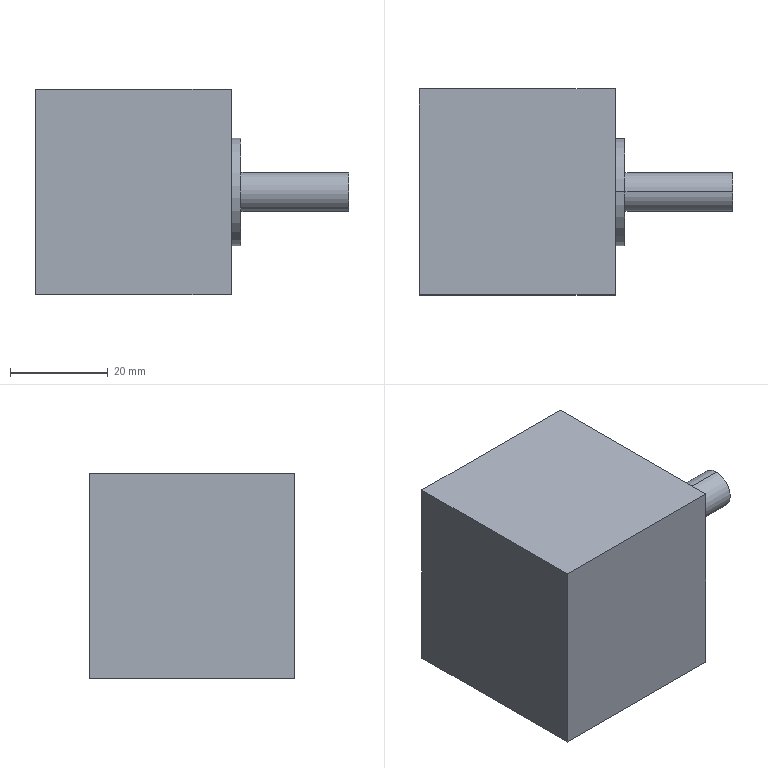Part | SolidWorks | features BaseBody 1 | 1 solid | 36 faces | box 64 x 42 x 42 mm | volume 72019 mm3 | cylinder 20 | plane 16 | commonest cylinder face diameters 3.4 x8 4.3 x8 8 x2 22 x2
STEP:
#1=CARTESIAN_POINT('',(-6.2,-15.5,17.65));
#2=VERTEX_POINT('',#1);
#3=CARTESIAN_POINT('',(-6.2,-15.5,13.35));
#4=VERTEX_POINT('',#3);
#5=CARTESIAN_POINT('',(-6.2,-15.5,15.5));
#6=DIRECTION('',(1.,0.,0.));
#7=DIRECTION('',(0.,0.,-1.));
#8=AXIS2_PLACEMENT_3D('',#5,#6,#7);
#9=CIRCLE('',#8,2.15);
#10=EDGE_CURVE('',#2,#4,#9,.T.);
#11=ORIENTED_EDGE('',*,*,#10,.F.);
#12=CARTESIAN_POINT('',(0.,-15.5,17.65));
#13=VERTEX_POINT('',#12);
#14=CARTESIAN_POINT('',(-6.2,-15.5,17.65));
#15=DIRECTION('',(1.,0.,0.));
#16=VECTOR('',#15,1000.);
#17=LINE('',#14,#16);
#18=EDGE_CURVE('',#2,#13,#17,.T.);
#19=ORIENTED_EDGE('',*,*,#18,.T.);
#20=CARTESIAN_POINT('',(0.,-15.5,13.35));
#21=VERTEX_POINT('',#20);
#22=CARTESIAN_POINT('',(0.,-15.5,15.5));
#23=DIRECTION('',(-1.,0.,0.));
#24=DIRECTION('',(0.,0.,-1.));
#25=AXIS2_PLACEMENT_3D('',#22,#23,#24);
#26=CIRCLE('',#25,2.15);
#27=EDGE_CURVE('',#21,#13,#26,.T.);
#28=ORIENTED_EDGE('',*,*,#27,.F.);
#29=CARTESIAN_POINT('',(-6.2,-15.5,13.35));
#30=DIRECTION('',(1.,0.,0.));
#31=VECTOR('',#30,1000.);
#32=LINE('',#29,#31);
#33=EDGE_CURVE('',#4,#21,#32,.T.);
#34=ORIENTED_EDGE('',*,*,#33,.F.);
#35=EDGE_LOOP('',(#11,#19,#28,#34));
#36=FACE_OUTER_BOUND('',#35,.T.);
#37=CARTESIAN_POINT('',(-6.2,-15.5,15.5));
#38=DIRECTION('',(1.,0.,0.));
#39=DIRECTION('',(0.,0.,-1.));
#40=AXIS2_PLACEMENT_3D('',#37,#38,#39);
#41=CYLINDRICAL_SURFACE('',#40,2.15);
#42=ADVANCED_FACE('',(#36),#41,.F.);
#43=CARTESIAN_POINT('',(0.,0.,11.));
#44=VERTEX_POINT('',#43);
#45=CARTESIAN_POINT('',(0.,0.,-11.));
#46=VERTEX_POINT('',#45);
#47=CARTESIAN_POINT('',(0.,0.,0.));
#48=DIRECTION('',(-1.,0.,0.));
#49=DIRECTION('',(0.,0.,-1.));
#50=AXIS2_PLACEMENT_3D('',#47,#48,#49);
#51=CIRCLE('',#50,11.);
#52=EDGE_CURVE('',#44,#46,#51,.T.);
#53=ORIENTED_EDGE('',*,*,#52,.F.);
#54=CARTESIAN_POINT('',(2.,0.,11.));
#55=VERTEX_POINT('',#54);
#56=CARTESIAN_POINT('',(0.,0.,11.));
#57=DIRECTION('',(1.,0.,0.));
#58=VECTOR('',#57,1000.);
#59=LINE('',#56,#58);
#60=EDGE_CURVE('',#44,#55,#59,.T.);
#61=ORIENTED_EDGE('',*,*,#60,.T.);
#62=CARTESIAN_POINT('',(2.,0.,-11.));
#63=VERTEX_POINT('',#62);
#64=CARTESIAN_POINT('',(2.,0.,0.));
#65=DIRECTION('',(-1.,0.,0.));
#66=DIRECTION('',(0.,0.,-1.));
#67=AXIS2_PLACEMENT_3D('',#64,#65,#66);
#68=CIRCLE('',#67,11.);
#69=EDGE_CURVE('',#55,#63,#68,.T.);
#70=ORIENTED_EDGE('',*,*,#69,.T.);
#71=CARTESIAN_POINT('',(0.,0.,-11.));
#72=DIRECTION('',(1.,0.,0.));
#73=VECTOR('',#72,1000.);
#74=LINE('',#71,#73);
#75=EDGE_CURVE('',#46,#63,#74,.T.);
#76=ORIENTED_EDGE('',*,*,#75,.F.);
#77=EDGE_LOOP('',(#53,#61,#70,#76));
#78=FACE_OUTER_BOUND('',#77,.T.);
#79=CARTESIAN_POINT('',(0.,0.,0.));
#80=DIRECTION('',(1.,0.,0.));
#81=DIRECTION('',(0.,0.,-1.));
#82=AXIS2_PLACEMENT_3D('',#79,#80,#81);
#83=CYLINDRICAL_SURFACE('',#82,11.);
#84=ADVANCED_FACE('',(#78),#83,.T.);
#85=CARTESIAN_POINT('',(-6.2,-15.5,-13.35));
#86=VERTEX_POINT('',#85);
#87=CARTESIAN_POINT('',(-6.2,-15.5,-17.65));
#88=VERTEX_POINT('',#87);
#89=CARTESIAN_POINT('',(-6.2,-15.5,-15.5));
#90=DIRECTION('',(1.,0.,0.));
#91=DIRECTION('',(0.,0.,-1.));
#92=AXIS2_PLACEMENT_3D('',#89,#90,#91);
#93=CIRCLE('',#92,2.15);
#94=EDGE_CURVE('',#86,#88,#93,.T.);
#95=ORIENTED_EDGE('',*,*,#94,.F.);
#96=CARTESIAN_POINT('',(0.,-15.5,-13.35));
#97=VERTEX_POINT('',#96);
#98=CARTESIAN_POINT('',(-6.2,-15.5,-13.35));
#99=DIRECTION('',(1.,0.,0.));
#100=VECTOR('',#99,1000.);
#101=LINE('',#98,#100);
#102=EDGE_CURVE('',#86,#97,#101,.T.);
#103=ORIENTED_EDGE('',*,*,#102,.T.);
#104=CARTESIAN_POINT('',(0.,-15.5,-17.65));
#105=VERTEX_POINT('',#104);
#106=CARTESIAN_POINT('',(0.,-15.5,-15.5));
#107=DIRECTION('',(-1.,0.,0.));
#108=DIRECTION('',(0.,0.,-1.));
#109=AXIS2_PLACEMENT_3D('',#106,#107,#108);
#110=CIRCLE('',#109,2.15);
#111=EDGE_CURVE('',#105,#97,#110,.T.);
#112=ORIENTED_EDGE('',*,*,#111,.F.);
#113=CARTESIAN_POINT('',(-6.2,-15.5,-17.65));
#114=DIRECTION('',(1.,0.,0.));
#115=VECTOR('',#114,1000.);
#116=LINE('',#113,#115);
#117=EDGE_CURVE('',#88,#105,#116,.T.);
#118=ORIENTED_EDGE('',*,*,#117,.F.);
#119=EDGE_LOOP('',(#95,#103,#112,#118));
#120=FACE_OUTER_BOUND('',#119,.T.);
#121=CARTESIAN_POINT('',(-6.2,-15.5,-15.5));
#122=DIRECTION('',(1.,0.,0.));
#123=DIRECTION('',(0.,0.,-1.));
#124=AXIS2_PLACEMENT_3D('',#121,#122,#123);
#125=CYLINDRICAL_SURFACE('',#124,2.15);
#126=ADVANCED_FACE('',(#120),#125,.F.);
#127=CARTESIAN_POINT('',(-6.2,15.5,17.65));
#128=VERTEX_POINT('',#127);
#129=CARTESIAN_POINT('',(-6.2,15.5,13.35));
#130=VERTEX_POINT('',#129);
#131=CARTESIAN_POINT('',(-6.2,15.5,15.5));
#132=DIRECTION('',(1.,0.,0.));
#133=DIRECTION('',(0.,0.,-1.));
#134=AXIS2_PLACEMENT_3D('',#131,#132,#133);
#135=CIRCLE('',#134,2.15);
#136=EDGE_CURVE('',#128,#130,#135,.T.);
#137=ORIENTED_EDGE('',*,*,#136,.F.);
#138=CARTESIAN_POINT('',(0.,15.5,17.65));
#139=VERTEX_POINT('',#138);
#140=CARTESIAN_POINT('',(-6.2,15.5,17.65));
#141=DIRECTION('',(1.,0.,0.));
#142=VECTOR('',#141,1000.);
#143=LINE('',#140,#142);
#144=EDGE_CURVE('',#128,#139,#143,.T.);
#145=ORIENTED_EDGE('',*,*,#144,.T.);
#146=CARTESIAN_POINT('',(0.,15.5,13.35));
#147=VERTEX_POINT('',#146);
#148=CARTESIAN_POINT('',(0.,15.5,15.5));
#149=DIRECTION('',(-1.,0.,0.));
#150=DIRECTION('',(0.,0.,-1.));
#151=AXIS2_PLACEMENT_3D('',#148,#149,#150);
#152=CIRCLE('',#151,2.15);
#153=EDGE_CURVE('',#147,#139,#152,.T.);
#154=ORIENTED_EDGE('',*,*,#153,.F.);
#155=CARTESIAN_POINT('',(-6.2,15.5,13.35));
#156=DIRECTION('',(1.,0.,0.));
#157=VECTOR('',#156,1000.);
#158=LINE('',#155,#157);
#159=EDGE_CURVE('',#130,#147,#158,.T.);
#160=ORIENTED_EDGE('',*,*,#159,.F.);
#161=EDGE_LOOP('',(#137,#145,#154,#160));
#162=FACE_OUTER_BOUND('',#161,.T.);
#163=CARTESIAN_POINT('',(-6.2,15.5,15.5));
#164=DIRECTION('',(1.,0.,0.));
#165=DIRECTION('',(0.,0.,-1.));
#166=AXIS2_PLACEMENT_3D('',#163,#164,#165);
#167=CYLINDRICAL_SURFACE('',#166,2.15);
#168=ADVANCED_FACE('',(#162),#167,.F.);
#169=CARTESIAN_POINT('',(-6.2,15.5,-13.35));
#170=VERTEX_POINT('',#169);
#171=CARTESIAN_POINT('',(-6.2,15.5,-17.65));
#172=VERTEX_POINT('',#171);
#173=CARTESIAN_POINT('',(-6.2,15.5,-15.5));
#174=DIRECTION('',(1.,0.,0.));
#175=DIRECTION('',(0.,0.,-1.));
#176=AXIS2_PLACEMENT_3D('',#173,#174,#175);
#177=CIRCLE('',#176,2.15);
#178=EDGE_CURVE('',#170,#172,#177,.T.);
#179=ORIENTED_EDGE('',*,*,#178,.F.);
#180=CARTESIAN_POINT('',(0.,15.5,-13.35));
#181=VERTEX_POINT('',#180);
#182=CARTESIAN_POINT('',(-6.2,15.5,-13.35));
#183=DIRECTION('',(1.,0.,0.));
#184=VECTOR('',#183,1000.);
#185=LINE('',#182,#184);
#186=EDGE_CURVE('',#170,#181,#185,.T.);
#187=ORIENTED_EDGE('',*,*,#186,.T.);
#188=CARTESIAN_POINT('',(0.,15.5,-17.65));
#189=VERTEX_POINT('',#188);
#190=CARTESIAN_POINT('',(0.,15.5,-15.5));
#191=DIRECTION('',(-1.,0.,0.));
#192=DIRECTION('',(0.,0.,-1.));
#193=AXIS2_PLACEMENT_3D('',#190,#191,#192);
#194=CIRCLE('',#193,2.15);
#195=EDGE_CURVE('',#189,#181,#194,.T.);
#196=ORIENTED_EDGE('',*,*,#195,.F.);
#197=CARTESIAN_POINT('',(-6.2,15.5,-17.65));
#198=DIRECTION('',(1.,0.,0.));
#199=VECTOR('',#198,1000.);
#200=LINE('',#197,#199);
#201=EDGE_CURVE('',#172,#189,#200,.T.);
#202=ORIENTED_EDGE('',*,*,#201,.F.);
#203=EDGE_LOOP('',(#179,#187,#196,#202));
#204=FACE_OUTER_BOUND('',#203,.T.);
#205=CARTESIAN_POINT('',(-6.2,15.5,-15.5));
#206=DIRECTION('',(1.,0.,0.));
#207=DIRECTION('',(0.,0.,-1.));
#208=AXIS2_PLACEMENT_3D('',#205,#206,#207);
#209=CYLINDRICAL_SURFACE('',#208,2.15);
#210=ADVANCED_FACE('',(#204),#209,.F.);
#211=CARTESIAN_POINT('',(-7.5,-15.5,17.2));
#212=VERTEX_POINT('',#211);
#213=CARTESIAN_POINT('',(-7.5,-15.5,13.8));
#214=VERTEX_POINT('',#213);
#215=CARTESIAN_POINT('',(-7.5,-15.5,15.5));
#216=DIRECTION('',(1.,0.,0.));
#217=DIRECTION('',(0.,0.,-1.));
#218=AXIS2_PLACEMENT_3D('',#215,#216,#217);
#219=CIRCLE('',#218,1.7);
#220=EDGE_CURVE('',#212,#214,#219,.T.);
#221=ORIENTED_EDGE('',*,*,#220,.F.);
#222=CARTESIAN_POINT('',(-6.2,-15.5,17.2));
#223=VERTEX_POINT('',#222);
#224=CARTESIAN_POINT('',(-7.5,-15.5,17.2));
#225=DIRECTION('',(1.,0.,0.));
#226=VECTOR('',#225,1000.);
#227=LINE('',#224,#226);
#228=EDGE_CURVE('',#212,#223,#227,.T.);
#229=ORIENTED_EDGE('',*,*,#228,.T.);
#230=CARTESIAN_POINT('',(-6.2,-15.5,13.8));
#231=VERTEX_POINT('',#230);
#232=CARTESIAN_POINT('',(-6.2,-15.5,15.5));
#233=DIRECTION('',(-1.,0.,0.));
#234=DIRECTION('',(0.,0.,-1.));
#235=AXIS2_PLACEMENT_3D('',#232,#233,#234);
#236=CIRCLE('',#235,1.7);
#237=EDGE_CURVE('',#231,#223,#236,.T.);
#238=ORIENTED_EDGE('',*,*,#237,.F.);
#239=CARTESIAN_POINT('',(-7.5,-15.5,13.8));
#240=DIRECTION('',(1.,0.,0.));
#241=VECTOR('',#240,1000.);
#242=LINE('',#239,#241);
#243=EDGE_CURVE('',#214,#231,#242,.T.);
#244=ORIENTED_EDGE('',*,*,#243,.F.);
#245=EDGE_LOOP('',(#221,#229,#238,#244));
#246=FACE_OUTER_BOUND('',#245,.T.);
#247=CARTESIAN_POINT('',(-7.5,-15.5,15.5));
#248=DIRECTION('',(1.,0.,0.));
#249=DIRECTION('',(0.,0.,-1.));
#250=AXIS2_PLACEMENT_3D('',#247,#248,#249);
#251=CYLINDRICAL_SURFACE('',#250,1.7);
#252=ADVANCED_FACE('',(#246),#251,.F.);
#253=CARTESIAN_POINT('',(2.,0.,4.));
#254=VERTEX_POINT('',#253);
#255=CARTESIAN_POINT('',(2.,0.,-4.));
#256=VERTEX_POINT('',#255);
#257=CARTESIAN_POINT('',(2.,0.,0.));
#258=DIRECTION('',(-1.,0.,0.));
#259=DIRECTION('',(0.,0.,-1.));
#260=AXIS2_PLACEMENT_3D('',#257,#258,#259);
#261=CIRCLE('',#260,4.);
#262=EDGE_CURVE('',#254,#256,#261,.T.);
#263=ORIENTED_EDGE('',*,*,#262,.F.);
#264=CARTESIAN_POINT('',(24.,0.,4.));
#265=VERTEX_POINT('',#264);
#266=CARTESIAN_POINT('',(2.,0.,4.));
#267=DIRECTION('',(1.,0.,0.));
#268=VECTOR('',#267,1000.);
#269=LINE('',#266,#268);
#270=EDGE_CURVE('',#254,#265,#269,.T.);
#271=ORIENTED_EDGE('',*,*,#270,.T.);
#272=CARTESIAN_POINT('',(24.,0.,-4.));
#273=VERTEX_POINT('',#272);
#274=CARTESIAN_POINT('',(24.,0.,0.));
#275=DIRECTION('',(-1.,0.,0.));
#276=DIRECTION('',(0.,0.,-1.));
#277=AXIS2_PLACEMENT_3D('',#274,#275,#276);
#278=CIRCLE('',#277,4.);
#279=EDGE_CURVE('',#265,#273,#278,.T.);
#280=ORIENTED_EDGE('',*,*,#279,.T.);
#281=CARTESIAN_POINT('',(2.,0.,-4.));
#282=DIRECTION('',(1.,0.,0.));
#283=VECTOR('',#282,1000.);
#284=LINE('',#281,#283);
#285=EDGE_CURVE('',#256,#273,#284,.T.);
#286=ORIENTED_EDGE('',*,*,#285,.F.);
#287=EDGE_LOOP('',(#263,#271,#280,#286));
#288=FACE_OUTER_BOUND('',#287,.T.);
#289=CARTESIAN_POINT('',(2.,0.,0.));
#290=DIRECTION('',(1.,0.,0.));
#291=DIRECTION('',(0.,0.,-1.));
#292=AXIS2_PLACEMENT_3D('',#289,#290,#291);
#293=CYLINDRICAL_SURFACE('',#292,4.);
#294=ADVANCED_FACE('',(#288),#293,.T.);
#295=CARTESIAN_POINT('',(-7.5,-15.5,-13.8));
#296=VERTEX_POINT('',#295);
#297=CARTESIAN_POINT('',(-7.5,-15.5,-17.2));
#298=VERTEX_POINT('',#297);
#299=CARTESIAN_POINT('',(-7.5,-15.5,-15.5));
#300=DIRECTION('',(1.,0.,0.));
#301=DIRECTION('',(0.,0.,-1.));
#302=AXIS2_PLACEMENT_3D('',#299,#300,#301);
#303=CIRCLE('',#302,1.7);
#304=EDGE_CURVE('',#296,#298,#303,.T.);
#305=ORIENTED_EDGE('',*,*,#304,.F.);
#306=CARTESIAN_POINT('',(-6.2,-15.5,-13.8));
#307=VERTEX_POINT('',#306);
#308=CARTESIAN_POINT('',(-7.5,-15.5,-13.8));
#309=DIRECTION('',(1.,0.,0.));
#310=VECTOR('',#309,1000.);
#311=LINE('',#308,#310);
#312=EDGE_CURVE('',#296,#307,#311,.T.);
#313=ORIENTED_EDGE('',*,*,#312,.T.);
#314=CARTESIAN_POINT('',(-6.2,-15.5,-17.2));
#315=VERTEX_POINT('',#314);
#316=CARTESIAN_POINT('',(-6.2,-15.5,-15.5));
#317=DIRECTION('',(-1.,0.,0.));
#318=DIRECTION('',(0.,0.,-1.));
#319=AXIS2_PLACEMENT_3D('',#316,#317,#318);
#320=CIRCLE('',#319,1.7);
#321=EDGE_CURVE('',#315,#307,#320,.T.);
#322=ORIENTED_EDGE('',*,*,#321,.F.);
#323=CARTESIAN_POINT('',(-7.5,-15.5,-17.2));
#324=DIRECTION('',(1.,0.,0.));
#325=VECTOR('',#324,1000.);
#326=LINE('',#323,#325);
#327=EDGE_CURVE('',#298,#315,#326,.T.);
#328=ORIENTED_EDGE('',*,*,#327,.F.);
#329=EDGE_LOOP('',(#305,#313,#322,#328));
#330=FACE_OUTER_BOUND('',#329,.T.);
#331=CARTESIAN_POINT('',(-7.5,-15.5,-15.5));
#332=DIRECTION('',(1.,0.,0.));
#333=DIRECTION('',(0.,0.,-1.));
#334=AXIS2_PLACEMENT_3D('',#331,#332,#333);
#335=CYLINDRICAL_SURFACE('',#334,1.7);
#336=ADVANCED_FACE('',(#330),#335,.F.);
#337=CARTESIAN_POINT('',(-7.5,15.5,17.2));
#338=VERTEX_POINT('',#337);
#339=CARTESIAN_POINT('',(-7.5,15.5,13.8));
#340=VERTEX_POINT('',#339);
#341=CARTESIAN_POINT('',(-7.5,15.5,15.5));
#342=DIRECTION('',(1.,0.,0.));
#343=DIRECTION('',(0.,0.,-1.));
#344=AXIS2_PLACEMENT_3D('',#341,#342,#343);
#345=CIRCLE('',#344,1.7);
#346=EDGE_CURVE('',#338,#340,#345,.T.);
#347=ORIENTED_EDGE('',*,*,#346,.F.);
#348=CARTESIAN_POINT('',(-6.2,15.5,17.2));
#349=VERTEX_POINT('',#348);
#350=CARTESIAN_POINT('',(-7.5,15.5,17.2));
#351=DIRECTION('',(1.,0.,0.));
#352=VECTOR('',#351,1000.);
#353=LINE('',#350,#352);
#354=EDGE_CURVE('',#338,#349,#353,.T.);
#355=ORIENTED_EDGE('',*,*,#354,.T.);
#356=CARTESIAN_POINT('',(-6.2,15.5,13.8));
#357=VERTEX_POINT('',#356);
#358=CARTESIAN_POINT('',(-6.2,15.5,15.5));
#359=DIRECTION('',(-1.,0.,0.));
#360=DIRECTION('',(0.,0.,-1.));
#361=AXIS2_PLACEMENT_3D('',#358,#359,#360);
#362=CIRCLE('',#361,1.7);
#363=EDGE_CURVE('',#357,#349,#362,.T.);
#364=ORIENTED_EDGE('',*,*,#363,.F.);
#365=CARTESIAN_POINT('',(-7.5,15.5,13.8));
#366=DIRECTION('',(1.,0.,0.));
#367=VECTOR('',#366,1000.);
#368=LINE('',#365,#367);
#369=EDGE_CURVE('',#340,#357,#368,.T.);
#370=ORIENTED_EDGE('',*,*,#369,.F.);
#371=EDGE_LOOP('',(#347,#355,#364,#370));
#372=FACE_OUTER_BOUND('',#371,.T.);
#373=CARTESIAN_POINT('',(-7.5,15.5,15.5));
#374=DIRECTION('',(1.,0.,0.));
#375=DIRECTION('',(0.,0.,-1.));
#376=AXIS2_PLACEMENT_3D('',#373,#374,#375);
#377=CYLINDRICAL_SURFACE('',#376,1.7);
#378=ADVANCED_FACE('',(#372),#377,.F.);
#379=CARTESIAN_POINT('',(-7.5,15.5,-13.8));
#380=VERTEX_POINT('',#379);
#381=CARTESIAN_POINT('',(-7.5,15.5,-17.2));
#382=VERTEX_POINT('',#381);
#383=CARTESIAN_POINT('',(-7.5,15.5,-15.5));
#384=DIRECTION('',(1.,0.,0.));
#385=DIRECTION('',(0.,0.,-1.));
#386=AXIS2_PLACEMENT_3D('',#383,#384,#385);
#387=CIRCLE('',#386,1.7);
#388=EDGE_CURVE('',#380,#382,#387,.T.);
#389=ORIENTED_EDGE('',*,*,#388,.F.);
#390=CARTESIAN_POINT('',(-6.2,15.5,-13.8));
#391=VERTEX_POINT('',#390);
#392=CARTESIAN_POINT('',(-7.5,15.5,-13.8));
#393=DIRECTION('',(1.,0.,0.));
#394=VECTOR('',#393,1000.);
#395=LINE('',#392,#394);
#396=EDGE_CURVE('',#380,#391,#395,.T.);
#397=ORIENTED_EDGE('',*,*,#396,.T.);
#398=CARTESIAN_POINT('',(-6.2,15.5,-17.2));
#399=VERTEX_POINT('',#398);
#400=CARTESIAN_POINT('',(-6.2,15.5,-15.5));
#401=DIRECTION('',(-1.,0.,0.));
#402=DIRECTION('',(0.,0.,-1.));
#403=AXIS2_PLACEMENT_3D('',#400,#401,#402);
#404=CIRCLE('',#403,1.7);
#405=EDGE_CURVE('',#399,#391,#404,.T.);
#406=ORIENTED_EDGE('',*,*,#405,.F.);
#407=CARTESIAN_POINT('',(-7.5,15.5,-17.2));
#408=DIRECTION('',(1.,0.,0.));
#409=VECTOR('',#408,1000.);
#410=LINE('',#407,#409);
#411=EDGE_CURVE('',#382,#399,#410,.T.);
#412=ORIENTED_EDGE('',*,*,#411,.F.);
#413=EDGE_LOOP('',(#389,#397,#406,#412));
#414=FACE_OUTER_BOUND('',#413,.T.);
#415=CARTESIAN_POINT('',(-7.5,15.5,-15.5));
#416=DIRECTION('',(1.,0.,0.));
#417=DIRECTION('',(0.,0.,-1.));
#418=AXIS2_PLACEMENT_3D('',#415,#416,#417);
#419=CYLINDRICAL_SURFACE('',#418,1.7);
#420=ADVANCED_FACE('',(#414),#419,.F.);
#421=CARTESIAN_POINT('',(-40.,21.,-21.));
#422=VERTEX_POINT('',#421);
#423=CARTESIAN_POINT('',(-40.,21.,21.));
#424=VERTEX_POINT('',#423);
#425=CARTESIAN_POINT('',(-40.,21.,-21.));
#426=DIRECTION('',(0.,0.,1.));
#427=VECTOR('',#426,1000.);
#428=LINE('',#425,#427);
#429=EDGE_CURVE('',#422,#424,#428,.T.);
#430=ORIENTED_EDGE('',*,*,#429,.F.);
#431=CARTESIAN_POINT('',(-40.,-21.,-21.));
#432=VERTEX_POINT('',#431);
#433=CARTESIAN_POINT('',(-40.,-21.,-21.));
#434=DIRECTION('',(0.,1.,0.));
#435=VECTOR('',#434,1000.);
#436=LINE('',#433,#435);
#437=EDGE_CURVE('',#432,#422,#436,.T.);
#438=ORIENTED_EDGE('',*,*,#437,.F.);
#439=CARTESIAN_POINT('',(-40.,-21.,21.));
#440=VERTEX_POINT('',#439);
#441=CARTESIAN_POINT('',(-40.,-21.,-21.));
#442=DIRECTION('',(0.,0.,-1.));
#443=VECTOR('',#442,1000.);
#444=LINE('',#441,#443);
#445=EDGE_CURVE('',#440,#432,#444,.T.);
#446=ORIENTED_EDGE('',*,*,#445,.F.);
#447=CARTESIAN_POINT('',(-40.,-21.,21.));
#448=DIRECTION('',(0.,-1.,0.));
#449=VECTOR('',#448,1000.);
#450=LINE('',#447,#449);
#451=EDGE_CURVE('',#424,#440,#450,.T.);
#452=ORIENTED_EDGE('',*,*,#451,.F.);
#453=EDGE_LOOP('',(#430,#438,#446,#452));
#454=FACE_OUTER_BOUND('',#453,.T.);
#455=CARTESIAN_POINT('',(-40.,-21.,-21.));
#456=DIRECTION('',(1.,0.,0.));
#457=DIRECTION('',(0.,0.,-1.));
#458=AXIS2_PLACEMENT_3D('',#455,#456,#457);
#459=PLANE('',#458);
#460=ADVANCED_FACE('',(#454),#459,.F.);
#461=CARTESIAN_POINT('',(0.,-21.,21.));
#462=VERTEX_POINT('',#461);
#463=CARTESIAN_POINT('',(0.,21.,21.));
#464=VERTEX_POINT('',#463);
#465=CARTESIAN_POINT('',(0.,-21.,21.));
#466=DIRECTION('',(0.,1.,0.));
#467=VECTOR('',#466,1000.);
#468=LINE('',#465,#467);
#469=EDGE_CURVE('',#462,#464,#468,.T.);
#470=ORIENTED_EDGE('',*,*,#469,.T.);
#471=CARTESIAN_POINT('',(-40.,21.,21.));
#472=DIRECTION('',(-1.,0.,0.));
#473=VECTOR('',#472,1000.);
#474=LINE('',#471,#473);
#475=EDGE_CURVE('',#464,#424,#474,.T.);
#476=ORIENTED_EDGE('',*,*,#475,.T.);
#477=ORIENTED_EDGE('',*,*,#451,.T.);
#478=CARTESIAN_POINT('',(-40.,-21.,21.));
#479=DIRECTION('',(1.,0.,0.));
#480=VECTOR('',#479,1000.);
#481=LINE('',#478,#480);
#482=EDGE_CURVE('',#440,#462,#481,.T.);
#483=ORIENTED_EDGE('',*,*,#482,.T.);
#484=EDGE_LOOP('',(#470,#476,#477,#483));
#485=FACE_OUTER_BOUND('',#484,.T.);
#486=CARTESIAN_POINT('',(-40.,-21.,21.));
#487=DIRECTION('',(0.,0.,1.));
#488=DIRECTION('',(1.,0.,0.));
#489=AXIS2_PLACEMENT_3D('',#486,#487,#488);
#490=PLANE('',#489);
#491=ADVANCED_FACE('',(#485),#490,.T.);
#492=ORIENTED_EDGE('',*,*,#475,.F.);
#493=CARTESIAN_POINT('',(0.,21.,-21.));
#494=VERTEX_POINT('',#493);
#495=CARTESIAN_POINT('',(0.,21.,-21.));
#496=DIRECTION('',(0.,0.,-1.));
#497=VECTOR('',#496,1000.);
#498=LINE('',#495,#497);
#499=EDGE_CURVE('',#464,#494,#498,.T.);
#500=ORIENTED_EDGE('',*,*,#499,.T.);
#501=CARTESIAN_POINT('',(-40.,21.,-21.));
#502=DIRECTION('',(-1.,0.,0.));
#503=VECTOR('',#502,1000.);
#504=LINE('',#501,#503);
#505=EDGE_CURVE('',#494,#422,#504,.T.);
#506=ORIENTED_EDGE('',*,*,#505,.T.);
#507=ORIENTED_EDGE('',*,*,#429,.T.);
#508=EDGE_LOOP('',(#492,#500,#506,#507));
#509=FACE_OUTER_BOUND('',#508,.T.);
#510=CARTESIAN_POINT('',(-40.,21.,-21.));
#511=DIRECTION('',(0.,1.,0.));
#512=DIRECTION('',(0.,0.,1.));
#513=AXIS2_PLACEMENT_3D('',#510,#511,#512);
#514=PLANE('',#513);
#515=ADVANCED_FACE('',(#509),#514,.T.);
#516=CARTESIAN_POINT('',(0.,-21.,-21.));
#517=VERTEX_POINT('',#516);
#518=CARTESIAN_POINT('',(0.,-21.,-21.));
#519=DIRECTION('',(0.,1.,0.));
#520=VECTOR('',#519,1000.);
#521=LINE('',#518,#520);
#522=EDGE_CURVE('',#517,#494,#521,.T.);
#523=ORIENTED_EDGE('',*,*,#522,.F.);
#524=CARTESIAN_POINT('',(-40.,-21.,-21.));
#525=DIRECTION('',(1.,0.,0.));
#526=VECTOR('',#525,1000.);
#527=LINE('',#524,#526);
#528=EDGE_CURVE('',#432,#517,#527,.T.);
#529=ORIENTED_EDGE('',*,*,#528,.F.);
#530=ORIENTED_EDGE('',*,*,#437,.T.);
#531=ORIENTED_EDGE('',*,*,#505,.F.);
#532=EDGE_LOOP('',(#523,#529,#530,#531));
#533=FACE_OUTER_BOUND('',#532,.T.);
#534=CARTESIAN_POINT('',(-40.,-21.,-21.));
#535=DIRECTION('',(0.,0.,1.));
#536=DIRECTION('',(1.,0.,0.));
#537=AXIS2_PLACEMENT_3D('',#534,#535,#536);
#538=PLANE('',#537);
#539=ADVANCED_FACE('',(#533),#538,.F.);
#540=ORIENTED_EDGE('',*,*,#482,.F.);
#541=ORIENTED_EDGE('',*,*,#445,.T.);
#542=ORIENTED_EDGE('',*,*,#528,.T.);
#543=CARTESIAN_POINT('',(0.,-21.,-21.));
#544=DIRECTION('',(0.,0.,-1.));
#545=VECTOR('',#544,1000.);
#546=LINE('',#543,#545);
#547=EDGE_CURVE('',#462,#517,#546,.T.);
#548=ORIENTED_EDGE('',*,*,#547,.F.);
#549=EDGE_LOOP('',(#540,#541,#542,#548));
#550=FACE_OUTER_BOUND('',#549,.T.);
#551=CARTESIAN_POINT('',(-40.,-21.,-21.));
#552=DIRECTION('',(0.,1.,0.));
#553=DIRECTION('',(0.,0.,1.));
#554=AXIS2_PLACEMENT_3D('',#551,#552,#553);
#555=PLANE('',#554);
#556=ADVANCED_FACE('',(#550),#555,.F.);
#557=ORIENTED_EDGE('',*,*,#27,.T.);
#558=CARTESIAN_POINT('',(0.,-15.5,15.5));
#559=DIRECTION('',(-1.,0.,0.));
#560=DIRECTION('',(0.,0.,-1.));
#561=AXIS2_PLACEMENT_3D('',#558,#559,#560);
#562=CIRCLE('',#561,2.15);
#563=EDGE_CURVE('',#13,#21,#562,.T.);
#564=ORIENTED_EDGE('',*,*,#563,.T.);
#565=EDGE_LOOP('',(#557,#564));
#566=FACE_BOUND('',#565,.T.);
#567=CARTESIAN_POINT('',(0.,0.,0.));
#568=DIRECTION('',(-1.,0.,0.));
#569=DIRECTION('',(0.,0.,-1.));
#570=AXIS2_PLACEMENT_3D('',#567,#568,#569);
#571=CIRCLE('',#570,11.);
#572=EDGE_CURVE('',#46,#44,#571,.T.);
#573=ORIENTED_EDGE('',*,*,#572,.T.);
#574=ORIENTED_EDGE('',*,*,#52,.T.);
#575=EDGE_LOOP('',(#573,#574));
#576=FACE_BOUND('',#575,.T.);
#577=ORIENTED_EDGE('',*,*,#111,.T.);
#578=CARTESIAN_POINT('',(0.,-15.5,-15.5));
#579=DIRECTION('',(-1.,0.,0.));
#580=DIRECTION('',(0.,0.,-1.));
#581=AXIS2_PLACEMENT_3D('',#578,#579,#580);
#582=CIRCLE('',#581,2.15);
#583=EDGE_CURVE('',#97,#105,#582,.T.);
#584=ORIENTED_EDGE('',*,*,#583,.T.);
#585=EDGE_LOOP('',(#577,#584));
#586=FACE_BOUND('',#585,.T.);
#587=ORIENTED_EDGE('',*,*,#153,.T.);
#588=CARTESIAN_POINT('',(0.,15.5,15.5));
#589=DIRECTION('',(-1.,0.,0.));
#590=DIRECTION('',(0.,0.,-1.));
#591=AXIS2_PLACEMENT_3D('',#588,#589,#590);
#592=CIRCLE('',#591,2.15);
#593=EDGE_CURVE('',#139,#147,#592,.T.);
#594=ORIENTED_EDGE('',*,*,#593,.T.);
#595=EDGE_LOOP('',(#587,#594));
#596=FACE_BOUND('',#595,.T.);
#597=ORIENTED_EDGE('',*,*,#195,.T.);
#598=CARTESIAN_POINT('',(0.,15.5,-15.5));
#599=DIRECTION('',(-1.,0.,0.));
#600=DIRECTION('',(0.,0.,-1.));
#601=AXIS2_PLACEMENT_3D('',#598,#599,#600);
#602=CIRCLE('',#601,2.15);
#603=EDGE_CURVE('',#181,#189,#602,.T.);
#604=ORIENTED_EDGE('',*,*,#603,.T.);
#605=EDGE_LOOP('',(#597,#604));
#606=FACE_BOUND('',#605,.T.);
#607=ORIENTED_EDGE('',*,*,#499,.F.);
#608=ORIENTED_EDGE('',*,*,#469,.F.);
#609=ORIENTED_EDGE('',*,*,#547,.T.);
#610=ORIENTED_EDGE('',*,*,#522,.T.);
#611=EDGE_LOOP('',(#607,#608,#609,#610));
#612=FACE_OUTER_BOUND('',#611,.T.);
#613=CARTESIAN_POINT('',(0.,-21.,-21.));
#614=DIRECTION('',(1.,0.,0.));
#615=DIRECTION('',(0.,0.,-1.));
#616=AXIS2_PLACEMENT_3D('',#613,#614,#615);
#617=PLANE('',#616);
#618=ADVANCED_FACE('',(#566,#576,#586,#596,#606,#612),#617,.T.);
#619=ORIENTED_EDGE('',*,*,#18,.F.);
#620=CARTESIAN_POINT('',(-6.2,-15.5,15.5));
#621=DIRECTION('',(1.,0.,0.));
#622=DIRECTION('',(0.,0.,-1.));
#623=AXIS2_PLACEMENT_3D('',#620,#621,#622);
#624=CIRCLE('',#623,2.15);
#625=EDGE_CURVE('',#4,#2,#624,.T.);
#626=ORIENTED_EDGE('',*,*,#625,.F.);
#627=ORIENTED_EDGE('',*,*,#33,.T.);
#628=ORIENTED_EDGE('',*,*,#563,.F.);
#629=EDGE_LOOP('',(#619,#626,#627,#628));
#630=FACE_OUTER_BOUND('',#629,.T.);
#631=CARTESIAN_POINT('',(-6.2,-15.5,15.5));
#632=DIRECTION('',(1.,0.,0.));
#633=DIRECTION('',(0.,0.,-1.));
#634=AXIS2_PLACEMENT_3D('',#631,#632,#633);
#635=CYLINDRICAL_SURFACE('',#634,2.15);
#636=ADVANCED_FACE('',(#630),#635,.F.);
#637=ORIENTED_EDGE('',*,*,#60,.F.);
#638=ORIENTED_EDGE('',*,*,#572,.F.);
#639=ORIENTED_EDGE('',*,*,#75,.T.);
#640=CARTESIAN_POINT('',(2.,0.,0.));
#641=DIRECTION('',(-1.,0.,0.));
#642=DIRECTION('',(0.,0.,-1.));
#643=AXIS2_PLACEMENT_3D('',#640,#641,#642);
#644=CIRCLE('',#643,11.);
#645=EDGE_CURVE('',#63,#55,#644,.T.);
#646=ORIENTED_EDGE('',*,*,#645,.T.);
#647=EDGE_LOOP('',(#637,#638,#639,#646));
#648=FACE_OUTER_BOUND('',#647,.T.);
#649=CARTESIAN_POINT('',(0.,0.,0.));
#650=DIRECTION('',(1.,0.,0.));
#651=DIRECTION('',(0.,0.,-1.));
#652=AXIS2_PLACEMENT_3D('',#649,#650,#651);
#653=CYLINDRICAL_SURFACE('',#652,11.);
#654=ADVANCED_FACE('',(#648),#653,.T.);
#655=ORIENTED_EDGE('',*,*,#102,.F.);
#656=CARTESIAN_POINT('',(-6.2,-15.5,-15.5));
#657=DIRECTION('',(1.,0.,0.));
#658=DIRECTION('',(0.,0.,-1.));
#659=AXIS2_PLACEMENT_3D('',#656,#657,#658);
#660=CIRCLE('',#659,2.15);
#661=EDGE_CURVE('',#88,#86,#660,.T.);
#662=ORIENTED_EDGE('',*,*,#661,.F.);
#663=ORIENTED_EDGE('',*,*,#117,.T.);
#664=ORIENTED_EDGE('',*,*,#583,.F.);
#665=EDGE_LOOP('',(#655,#662,#663,#664));
#666=FACE_OUTER_BOUND('',#665,.T.);
#667=CARTESIAN_POINT('',(-6.2,-15.5,-15.5));
#668=DIRECTION('',(1.,0.,0.));
#669=DIRECTION('',(0.,0.,-1.));
#670=AXIS2_PLACEMENT_3D('',#667,#668,#669);
#671=CYLINDRICAL_SURFACE('',#670,2.15);
#672=ADVANCED_FACE('',(#666),#671,.F.);
#673=ORIENTED_EDGE('',*,*,#144,.F.);
#674=CARTESIAN_POINT('',(-6.2,15.5,15.5));
#675=DIRECTION('',(1.,0.,0.));
#676=DIRECTION('',(0.,0.,-1.));
#677=AXIS2_PLACEMENT_3D('',#674,#675,#676);
#678=CIRCLE('',#677,2.15);
#679=EDGE_CURVE('',#130,#128,#678,.T.);
#680=ORIENTED_EDGE('',*,*,#679,.F.);
#681=ORIENTED_EDGE('',*,*,#159,.T.);
#682=ORIENTED_EDGE('',*,*,#593,.F.);
#683=EDGE_LOOP('',(#673,#680,#681,#682));
#684=FACE_OUTER_BOUND('',#683,.T.);
#685=CARTESIAN_POINT('',(-6.2,15.5,15.5));
#686=DIRECTION('',(1.,0.,0.));
#687=DIRECTION('',(0.,0.,-1.));
#688=AXIS2_PLACEMENT_3D('',#685,#686,#687);
#689=CYLINDRICAL_SURFACE('',#688,2.15);
#690=ADVANCED_FACE('',(#684),#689,.F.);
#691=ORIENTED_EDGE('',*,*,#186,.F.);
#692=CARTESIAN_POINT('',(-6.2,15.5,-15.5));
#693=DIRECTION('',(1.,0.,0.));
#694=DIRECTION('',(0.,0.,-1.));
#695=AXIS2_PLACEMENT_3D('',#692,#693,#694);
#696=CIRCLE('',#695,2.15);
#697=EDGE_CURVE('',#172,#170,#696,.T.);
#698=ORIENTED_EDGE('',*,*,#697,.F.);
#699=ORIENTED_EDGE('',*,*,#201,.T.);
#700=ORIENTED_EDGE('',*,*,#603,.F.);
#701=EDGE_LOOP('',(#691,#698,#699,#700));
#702=FACE_OUTER_BOUND('',#701,.T.);
#703=CARTESIAN_POINT('',(-6.2,15.5,-15.5));
#704=DIRECTION('',(1.,0.,0.));
#705=DIRECTION('',(0.,0.,-1.));
#706=AXIS2_PLACEMENT_3D('',#703,#704,#705);
#707=CYLINDRICAL_SURFACE('',#706,2.15);
#708=ADVANCED_FACE('',(#702),#707,.F.);
#709=ORIENTED_EDGE('',*,*,#237,.T.);
#710=CARTESIAN_POINT('',(-6.2,-15.5,15.5));
#711=DIRECTION('',(-1.,0.,0.));
#712=DIRECTION('',(0.,0.,-1.));
#713=AXIS2_PLACEMENT_3D('',#710,#711,#712);
#714=CIRCLE('',#713,1.7);
#715=EDGE_CURVE('',#223,#231,#714,.T.);
#716=ORIENTED_EDGE('',*,*,#715,.T.);
#717=EDGE_LOOP('',(#709,#716));
#718=FACE_BOUND('',#717,.T.);
#719=ORIENTED_EDGE('',*,*,#625,.T.);
#720=ORIENTED_EDGE('',*,*,#10,.T.);
#721=EDGE_LOOP('',(#719,#720));
#722=FACE_OUTER_BOUND('',#721,.T.);
#723=CARTESIAN_POINT('',(-6.2,-15.5,15.5));
#724=DIRECTION('',(1.,0.,0.));
#725=DIRECTION('',(0.,0.,-1.));
#726=AXIS2_PLACEMENT_3D('',#723,#724,#725);
#727=PLANE('',#726);
#728=ADVANCED_FACE('',(#718,#722),#727,.T.);
#729=CARTESIAN_POINT('',(2.,0.,0.));
#730=DIRECTION('',(-1.,0.,0.));
#731=DIRECTION('',(0.,0.,-1.));
#732=AXIS2_PLACEMENT_3D('',#729,#730,#731);
#733=CIRCLE('',#732,4.);
#734=EDGE_CURVE('',#256,#254,#733,.T.);
#735=ORIENTED_EDGE('',*,*,#734,.T.);
#736=ORIENTED_EDGE('',*,*,#262,.T.);
#737=EDGE_LOOP('',(#735,#736));
#738=FACE_BOUND('',#737,.T.);
#739=ORIENTED_EDGE('',*,*,#645,.F.);
#740=ORIENTED_EDGE('',*,*,#69,.F.);
#741=EDGE_LOOP('',(#739,#740));
#742=FACE_OUTER_BOUND('',#741,.T.);
#743=CARTESIAN_POINT('',(2.,0.,0.));
#744=DIRECTION('',(1.,0.,0.));
#745=DIRECTION('',(0.,0.,-1.));
#746=AXIS2_PLACEMENT_3D('',#743,#744,#745);
#747=PLANE('',#746);
#748=ADVANCED_FACE('',(#738,#742),#747,.T.);
#749=ORIENTED_EDGE('',*,*,#321,.T.);
#750=CARTESIAN_POINT('',(-6.2,-15.5,-15.5));
#751=DIRECTION('',(-1.,0.,0.));
#752=DIRECTION('',(0.,0.,-1.));
#753=AXIS2_PLACEMENT_3D('',#750,#751,#752);
#754=CIRCLE('',#753,1.7);
#755=EDGE_CURVE('',#307,#315,#754,.T.);
#756=ORIENTED_EDGE('',*,*,#755,.T.);
#757=EDGE_LOOP('',(#749,#756));
#758=FACE_BOUND('',#757,.T.);
#759=ORIENTED_EDGE('',*,*,#661,.T.);
#760=ORIENTED_EDGE('',*,*,#94,.T.);
#761=EDGE_LOOP('',(#759,#760));
#762=FACE_OUTER_BOUND('',#761,.T.);
#763=CARTESIAN_POINT('',(-6.2,-15.5,-15.5));
#764=DIRECTION('',(1.,0.,0.));
#765=DIRECTION('',(0.,0.,-1.));
#766=AXIS2_PLACEMENT_3D('',#763,#764,#765);
#767=PLANE('',#766);
#768=ADVANCED_FACE('',(#758,#762),#767,.T.);
#769=ORIENTED_EDGE('',*,*,#363,.T.);
#770=CARTESIAN_POINT('',(-6.2,15.5,15.5));
#771=DIRECTION('',(-1.,0.,0.));
#772=DIRECTION('',(0.,0.,-1.));
#773=AXIS2_PLACEMENT_3D('',#770,#771,#772);
#774=CIRCLE('',#773,1.7);
#775=EDGE_CURVE('',#349,#357,#774,.T.);
#776=ORIENTED_EDGE('',*,*,#775,.T.);
#777=EDGE_LOOP('',(#769,#776));
#778=FACE_BOUND('',#777,.T.);
#779=ORIENTED_EDGE('',*,*,#679,.T.);
#780=ORIENTED_EDGE('',*,*,#136,.T.);
#781=EDGE_LOOP('',(#779,#780));
#782=FACE_OUTER_BOUND('',#781,.T.);
#783=CARTESIAN_POINT('',(-6.2,15.5,15.5));
#784=DIRECTION('',(1.,0.,0.));
#785=DIRECTION('',(0.,0.,-1.));
#786=AXIS2_PLACEMENT_3D('',#783,#784,#785);
#787=PLANE('',#786);
#788=ADVANCED_FACE('',(#778,#782),#787,.T.);
#789=ORIENTED_EDGE('',*,*,#405,.T.);
#790=CARTESIAN_POINT('',(-6.2,15.5,-15.5));
#791=DIRECTION('',(-1.,0.,0.));
#792=DIRECTION('',(0.,0.,-1.));
#793=AXIS2_PLACEMENT_3D('',#790,#791,#792);
#794=CIRCLE('',#793,1.7);
#795=EDGE_CURVE('',#391,#399,#794,.T.);
#796=ORIENTED_EDGE('',*,*,#795,.T.);
#797=EDGE_LOOP('',(#789,#796));
#798=FACE_BOUND('',#797,.T.);
#799=ORIENTED_EDGE('',*,*,#697,.T.);
#800=ORIENTED_EDGE('',*,*,#178,.T.);
#801=EDGE_LOOP('',(#799,#800));
#802=FACE_OUTER_BOUND('',#801,.T.);
#803=CARTESIAN_POINT('',(-6.2,15.5,-15.5));
#804=DIRECTION('',(1.,0.,0.));
#805=DIRECTION('',(0.,0.,-1.));
#806=AXIS2_PLACEMENT_3D('',#803,#804,#805);
#807=PLANE('',#806);
#808=ADVANCED_FACE('',(#798,#802),#807,.T.);
#809=ORIENTED_EDGE('',*,*,#228,.F.);
#810=CARTESIAN_POINT('',(-7.5,-15.5,15.5));
#811=DIRECTION('',(1.,0.,0.));
#812=DIRECTION('',(0.,0.,-1.));
#813=AXIS2_PLACEMENT_3D('',#810,#811,#812);
#814=CIRCLE('',#813,1.7);
#815=EDGE_CURVE('',#214,#212,#814,.T.);
#816=ORIENTED_EDGE('',*,*,#815,.F.);
#817=ORIENTED_EDGE('',*,*,#243,.T.);
#818=ORIENTED_EDGE('',*,*,#715,.F.);
#819=EDGE_LOOP('',(#809,#816,#817,#818));
#820=FACE_OUTER_BOUND('',#819,.T.);
#821=CARTESIAN_POINT('',(-7.5,-15.5,15.5));
#822=DIRECTION('',(1.,0.,0.));
#823=DIRECTION('',(0.,0.,-1.));
#824=AXIS2_PLACEMENT_3D('',#821,#822,#823);
#825=CYLINDRICAL_SURFACE('',#824,1.7);
#826=ADVANCED_FACE('',(#820),#825,.F.);
#827=ORIENTED_EDGE('',*,*,#270,.F.);
#828=ORIENTED_EDGE('',*,*,#734,.F.);
#829=ORIENTED_EDGE('',*,*,#285,.T.);
#830=CARTESIAN_POINT('',(24.,0.,0.));
#831=DIRECTION('',(-1.,0.,0.));
#832=DIRECTION('',(0.,0.,-1.));
#833=AXIS2_PLACEMENT_3D('',#830,#831,#832);
#834=CIRCLE('',#833,4.);
#835=EDGE_CURVE('',#273,#265,#834,.T.);
#836=ORIENTED_EDGE('',*,*,#835,.T.);
#837=EDGE_LOOP('',(#827,#828,#829,#836));
#838=FACE_OUTER_BOUND('',#837,.T.);
#839=CARTESIAN_POINT('',(2.,0.,0.));
#840=DIRECTION('',(1.,0.,0.));
#841=DIRECTION('',(0.,0.,-1.));
#842=AXIS2_PLACEMENT_3D('',#839,#840,#841);
#843=CYLINDRICAL_SURFACE('',#842,4.);
#844=ADVANCED_FACE('',(#838),#843,.T.);
#845=ORIENTED_EDGE('',*,*,#312,.F.);
#846=CARTESIAN_POINT('',(-7.5,-15.5,-15.5));
#847=DIRECTION('',(1.,0.,0.));
#848=DIRECTION('',(0.,0.,-1.));
#849=AXIS2_PLACEMENT_3D('',#846,#847,#848);
#850=CIRCLE('',#849,1.7);
#851=EDGE_CURVE('',#298,#296,#850,.T.);
#852=ORIENTED_EDGE('',*,*,#851,.F.);
#853=ORIENTED_EDGE('',*,*,#327,.T.);
#854=ORIENTED_EDGE('',*,*,#755,.F.);
#855=EDGE_LOOP('',(#845,#852,#853,#854));
#856=FACE_OUTER_BOUND('',#855,.T.);
#857=CARTESIAN_POINT('',(-7.5,-15.5,-15.5));
#858=DIRECTION('',(1.,0.,0.));
#859=DIRECTION('',(0.,0.,-1.));
#860=AXIS2_PLACEMENT_3D('',#857,#858,#859);
#861=CYLINDRICAL_SURFACE('',#860,1.7);
#862=ADVANCED_FACE('',(#856),#861,.F.);
#863=ORIENTED_EDGE('',*,*,#354,.F.);
#864=CARTESIAN_POINT('',(-7.5,15.5,15.5));
#865=DIRECTION('',(1.,0.,0.));
#866=DIRECTION('',(0.,0.,-1.));
#867=AXIS2_PLACEMENT_3D('',#864,#865,#866);
#868=CIRCLE('',#867,1.7);
#869=EDGE_CURVE('',#340,#338,#868,.T.);
#870=ORIENTED_EDGE('',*,*,#869,.F.);
#871=ORIENTED_EDGE('',*,*,#369,.T.);
#872=ORIENTED_EDGE('',*,*,#775,.F.);
#873=EDGE_LOOP('',(#863,#870,#871,#872));
#874=FACE_OUTER_BOUND('',#873,.T.);
#875=CARTESIAN_POINT('',(-7.5,15.5,15.5));
#876=DIRECTION('',(1.,0.,0.));
#877=DIRECTION('',(0.,0.,-1.));
#878=AXIS2_PLACEMENT_3D('',#875,#876,#877);
#879=CYLINDRICAL_SURFACE('',#878,1.7);
#880=ADVANCED_FACE('',(#874),#879,.F.);
#881=ORIENTED_EDGE('',*,*,#396,.F.);
#882=CARTESIAN_POINT('',(-7.5,15.5,-15.5));
#883=DIRECTION('',(1.,0.,0.));
#884=DIRECTION('',(0.,0.,-1.));
#885=AXIS2_PLACEMENT_3D('',#882,#883,#884);
#886=CIRCLE('',#885,1.7);
#887=EDGE_CURVE('',#382,#380,#886,.T.);
#888=ORIENTED_EDGE('',*,*,#887,.F.);
#889=ORIENTED_EDGE('',*,*,#411,.T.);
#890=ORIENTED_EDGE('',*,*,#795,.F.);
#891=EDGE_LOOP('',(#881,#888,#889,#890));
#892=FACE_OUTER_BOUND('',#891,.T.);
#893=CARTESIAN_POINT('',(-7.5,15.5,-15.5));
#894=DIRECTION('',(1.,0.,0.));
#895=DIRECTION('',(0.,0.,-1.));
#896=AXIS2_PLACEMENT_3D('',#893,#894,#895);
#897=CYLINDRICAL_SURFACE('',#896,1.7);
#898=ADVANCED_FACE('',(#892),#897,.F.);
#899=ORIENTED_EDGE('',*,*,#815,.T.);
#900=ORIENTED_EDGE('',*,*,#220,.T.);
#901=EDGE_LOOP('',(#899,#900));
#902=FACE_OUTER_BOUND('',#901,.T.);
#903=CARTESIAN_POINT('',(-7.5,-15.5,15.5));
#904=DIRECTION('',(1.,0.,0.));
#905=DIRECTION('',(0.,0.,-1.));
#906=AXIS2_PLACEMENT_3D('',#903,#904,#905);
#907=PLANE('',#906);
#908=ADVANCED_FACE('',(#902),#907,.T.);
#909=ORIENTED_EDGE('',*,*,#835,.F.);
#910=ORIENTED_EDGE('',*,*,#279,.F.);
#911=EDGE_LOOP('',(#909,#910));
#912=FACE_OUTER_BOUND('',#911,.T.);
#913=CARTESIAN_POINT('',(24.,0.,0.));
#914=DIRECTION('',(1.,0.,0.));
#915=DIRECTION('',(0.,0.,-1.));
#916=AXIS2_PLACEMENT_3D('',#913,#914,#915);
#917=PLANE('',#916);
#918=ADVANCED_FACE('',(#912),#917,.T.);
#919=ORIENTED_EDGE('',*,*,#851,.T.);
#920=ORIENTED_EDGE('',*,*,#304,.T.);
#921=EDGE_LOOP('',(#919,#920));
#922=FACE_OUTER_BOUND('',#921,.T.);
#923=CARTESIAN_POINT('',(-7.5,-15.5,-15.5));
#924=DIRECTION('',(1.,0.,0.));
#925=DIRECTION('',(0.,0.,-1.));
#926=AXIS2_PLACEMENT_3D('',#923,#924,#925);
#927=PLANE('',#926);
#928=ADVANCED_FACE('',(#922),#927,.T.);
#929=ORIENTED_EDGE('',*,*,#869,.T.);
#930=ORIENTED_EDGE('',*,*,#346,.T.);
#931=EDGE_LOOP('',(#929,#930));
#932=FACE_OUTER_BOUND('',#931,.T.);
#933=CARTESIAN_POINT('',(-7.5,15.5,15.5));
#934=DIRECTION('',(1.,0.,0.));
#935=DIRECTION('',(0.,0.,-1.));
#936=AXIS2_PLACEMENT_3D('',#933,#934,#935);
#937=PLANE('',#936);
#938=ADVANCED_FACE('',(#932),#937,.T.);
#939=ORIENTED_EDGE('',*,*,#887,.T.);
#940=ORIENTED_EDGE('',*,*,#388,.T.);
#941=EDGE_LOOP('',(#939,#940));
#942=FACE_OUTER_BOUND('',#941,.T.);
#943=CARTESIAN_POINT('',(-7.5,15.5,-15.5));
#944=DIRECTION('',(1.,0.,0.));
#945=DIRECTION('',(0.,0.,-1.));
#946=AXIS2_PLACEMENT_3D('',#943,#944,#945);
#947=PLANE('',#946);
#948=ADVANCED_FACE('',(#942),#947,.T.);
#949=CLOSED_SHELL('',(#42,#84,#126,#168,#210,#252,#294,#336,#378,#420,#460,#491,#515,#539,#556,#618,#636,#654,#672,#690,#708,#728,#748,#768,#788,#808,#826,#844,#862,#880,#898,#908,#918,#928,#938,#948));
#950=MANIFOLD_SOLID_BREP('',#949);
#951=CARTESIAN_POINT('',(0.,0.,0.));
#952=DIRECTION('',(0.,0.,1.));
#953=DIRECTION('',(1.,0.,0.));
#954=AXIS2_PLACEMENT_3D('',#951,#952,#953);
#955=(LENGTH_UNIT()NAMED_UNIT(*)SI_UNIT(.MILLI.,.METRE.));
#956=UNCERTAINTY_MEASURE_WITH_UNIT(LENGTH_MEASURE(0.00001),#955,'','');
#957=(NAMED_UNIT(*)PLANE_ANGLE_UNIT()SI_UNIT($,.RADIAN.));
#958=(NAMED_UNIT(*)SI_UNIT($,.STERADIAN.)SOLID_ANGLE_UNIT());
#959=(GEOMETRIC_REPRESENTATION_CONTEXT(3)GLOBAL_UNCERTAINTY_ASSIGNED_CONTEXT((#956))GLOBAL_UNIT_ASSIGNED_CONTEXT((#955,#957,#958))REPRESENTATION_CONTEXT('',''));
#960=ADVANCED_BREP_SHAPE_REPRESENTATION('',(#950,#954),#959);